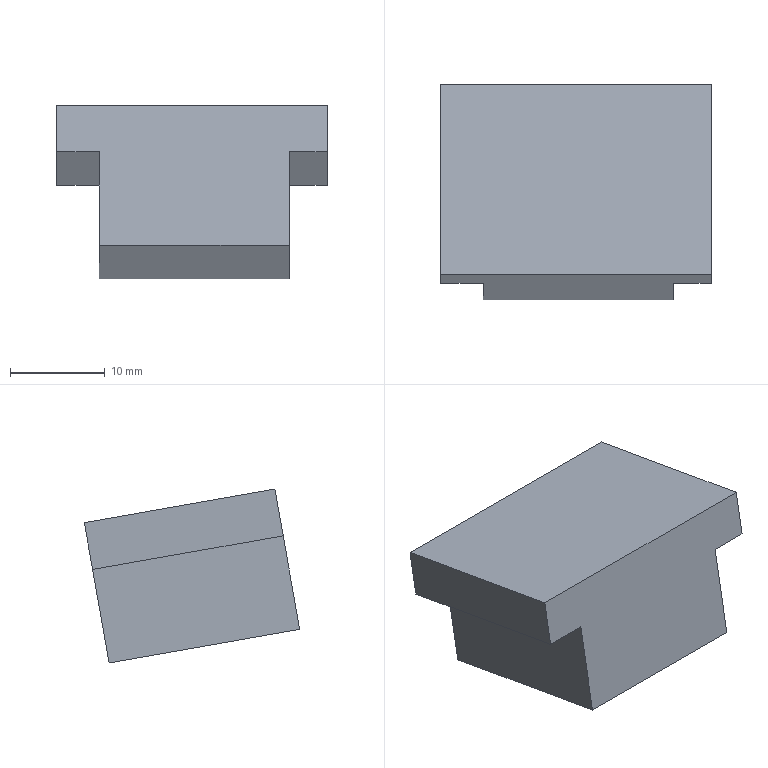Part | STEP file | 1 solid | 10 faces | box 28.5 x 22.681 x 18.312 mm | volume 6982 mm3 | plane 10
STEP:
#1=CARTESIAN_POINT('',(0.,0.,0.));
#2=DIRECTION('',(0.,0.,1.));
#3=DIRECTION('',(1.,0.,0.));
#4=AXIS2_PLACEMENT_3D('',#1,#2,#3);
#5=CARTESIAN_POINT('',(-28.862,49.056,-74.558));
#6=VERTEX_POINT('',#5);
#7=CARTESIAN_POINT('',(-32.862,49.056,-74.558));
#8=VERTEX_POINT('',#7);
#9=CARTESIAN_POINT('',(-43.112,49.056,-74.558));
#10=DIRECTION('',(-1.,0.,0.));
#11=VECTOR('',#10,1.);
#12=LINE('',#9,#11);
#13=CARTESIAN_POINT('',(-42.862,55.937,-75.771));
#14=DIRECTION('',(0.,-0.1736,-0.9848));
#15=DIRECTION('',(0.,0.9848,-0.1736));
#16=AXIS2_PLACEMENT_3D('',#13,#14,#15);
#17=PLANE('',#16);
#18=CARTESIAN_POINT('',(-6.987,-0.25));
#19=DIRECTION('',(0.,-1.));
#20=VECTOR('',#19,1.);
#21=LINE('',#18,#20);
#22=(GEOMETRIC_REPRESENTATION_CONTEXT(2)PARAMETRIC_REPRESENTATION_CONTEXT()REPRESENTATION_CONTEXT('',''));
#23=DEFINITIONAL_REPRESENTATION('',(#21),#22);
#24=PCURVE('',#17,#23);
#25=CARTESIAN_POINT('',(-43.112,49.924,-69.634));
#26=DIRECTION('',(0.,-0.9848,0.1736));
#27=DIRECTION('',(0.,-0.1736,-0.9848));
#28=AXIS2_PLACEMENT_3D('',#25,#26,#27);
#29=PLANE('',#28);
#30=CARTESIAN_POINT('',(5.,0.));
#31=DIRECTION('',(0.,-1.));
#32=VECTOR('',#31,1.);
#33=LINE('',#30,#32);
#34=(GEOMETRIC_REPRESENTATION_CONTEXT(2)PARAMETRIC_REPRESENTATION_CONTEXT()REPRESENTATION_CONTEXT('',''));
#35=DEFINITIONAL_REPRESENTATION('',(#33),#34);
#36=PCURVE('',#29,#35);
#37=SURFACE_CURVE('',#12,(#24,#36),.PCURVE_S1.);
#38=EDGE_CURVE('',#6,#8,#37,.T.);
#39=ORIENTED_EDGE('',*,*,#38,.T.);
#40=CARTESIAN_POINT('',(-32.862,69.132,-78.097));
#41=VERTEX_POINT('',#40);
#42=CARTESIAN_POINT('',(-32.862,4.542,-66.709));
#43=DIRECTION('',(0.,0.9848,-0.1736));
#44=VECTOR('',#43,1.);
#45=LINE('',#42,#44);
#46=CARTESIAN_POINT('',(-52.187,10.));
#47=DIRECTION('',(1.,0.));
#48=VECTOR('',#47,1.);
#49=LINE('',#46,#48);
#50=(GEOMETRIC_REPRESENTATION_CONTEXT(2)PARAMETRIC_REPRESENTATION_CONTEXT()REPRESENTATION_CONTEXT('',''));
#51=DEFINITIONAL_REPRESENTATION('',(#49),#50);
#52=PCURVE('',#17,#51);
#53=CARTESIAN_POINT('',(-32.862,0.,-92.47));
#54=DIRECTION('',(1.,0.,0.));
#55=DIRECTION('',(0.,0.,-1.));
#56=AXIS2_PLACEMENT_3D('',#53,#54,#55);
#57=PLANE('',#56);
#58=CARTESIAN_POINT('',(-25.762,4.542));
#59=DIRECTION('',(0.1736,0.9848));
#60=VECTOR('',#59,1.);
#61=LINE('',#58,#60);
#62=(GEOMETRIC_REPRESENTATION_CONTEXT(2)PARAMETRIC_REPRESENTATION_CONTEXT()REPRESENTATION_CONTEXT('',''));
#63=DEFINITIONAL_REPRESENTATION('',(#61),#62);
#64=PCURVE('',#57,#63);
#65=SURFACE_CURVE('',#45,(#52,#64),.PCURVE_S1.);
#66=EDGE_CURVE('',#8,#41,#65,.T.);
#67=ORIENTED_EDGE('',*,*,#66,.T.);
#68=CARTESIAN_POINT('',(-28.862,69.132,-78.097));
#69=VERTEX_POINT('',#68);
#70=CARTESIAN_POINT('',(-43.112,69.132,-78.097));
#71=DIRECTION('',(-1.,0.,0.));
#72=VECTOR('',#71,1.);
#73=LINE('',#70,#72);
#74=CARTESIAN_POINT('',(13.398,-0.25));
#75=DIRECTION('',(0.,-1.));
#76=VECTOR('',#75,1.);
#77=LINE('',#74,#76);
#78=(GEOMETRIC_REPRESENTATION_CONTEXT(2)PARAMETRIC_REPRESENTATION_CONTEXT()REPRESENTATION_CONTEXT('',''));
#79=DEFINITIONAL_REPRESENTATION('',(#77),#78);
#80=PCURVE('',#17,#79);
#81=CARTESIAN_POINT('',(-43.112,70.,-73.173));
#82=DIRECTION('',(0.,0.9848,-0.1736));
#83=DIRECTION('',(0.,0.1736,0.9848));
#84=AXIS2_PLACEMENT_3D('',#81,#82,#83);
#85=PLANE('',#84);
#86=CARTESIAN_POINT('',(-5.,0.));
#87=DIRECTION('',(0.,-1.));
#88=VECTOR('',#87,1.);
#89=LINE('',#86,#88);
#90=(GEOMETRIC_REPRESENTATION_CONTEXT(2)PARAMETRIC_REPRESENTATION_CONTEXT()REPRESENTATION_CONTEXT('',''));
#91=DEFINITIONAL_REPRESENTATION('',(#89),#90);
#92=PCURVE('',#85,#91);
#93=SURFACE_CURVE('',#73,(#80,#92),.PCURVE_S1.);
#94=EDGE_CURVE('',#69,#41,#93,.T.);
#95=ORIENTED_EDGE('',*,*,#94,.F.);
#96=CARTESIAN_POINT('',(-28.862,55.937,-75.771));
#97=DIRECTION('',(0.,-0.9848,0.1736));
#98=VECTOR('',#97,1.);
#99=LINE('',#96,#98);
#100=CARTESIAN_POINT('',(0.,14.));
#101=DIRECTION('',(-1.,0.));
#102=VECTOR('',#101,1.);
#103=LINE('',#100,#102);
#104=(GEOMETRIC_REPRESENTATION_CONTEXT(2)PARAMETRIC_REPRESENTATION_CONTEXT()REPRESENTATION_CONTEXT('',''));
#105=DEFINITIONAL_REPRESENTATION('',(#103),#104);
#106=PCURVE('',#17,#105);
#107=CARTESIAN_POINT('',(-28.862,57.5,-78.156));
#108=DIRECTION('',(1.,0.,0.));
#109=DIRECTION('',(0.,0.,-1.));
#110=AXIS2_PLACEMENT_3D('',#107,#108,#109);
#111=PLANE('',#110);
#112=CARTESIAN_POINT('',(-2.385,-1.563));
#113=DIRECTION('',(-0.1736,-0.9848));
#114=VECTOR('',#113,1.);
#115=LINE('',#112,#114);
#116=(GEOMETRIC_REPRESENTATION_CONTEXT(2)PARAMETRIC_REPRESENTATION_CONTEXT()REPRESENTATION_CONTEXT('',''));
#117=DEFINITIONAL_REPRESENTATION('',(#115),#116);
#118=PCURVE('',#111,#117);
#119=SURFACE_CURVE('',#99,(#106,#118),.PCURVE_S1.);
#120=EDGE_CURVE('',#69,#6,#119,.T.);
#121=ORIENTED_EDGE('',*,*,#120,.T.);
#122=EDGE_LOOP('',(#39,#67,#95,#121));
#123=FACE_BOUND('',#122,.T.);
#124=ADVANCED_FACE('',(#123),#17,.T.);
#125=CARTESIAN_POINT('',(-52.862,69.132,-78.097));
#126=VERTEX_POINT('',#125);
#127=CARTESIAN_POINT('',(-57.362,69.132,-78.097));
#128=VERTEX_POINT('',#127);
#129=CARTESIAN_POINT('',(-43.112,69.132,-78.097));
#130=DIRECTION('',(-1.,0.,0.));
#131=VECTOR('',#130,1.);
#132=LINE('',#129,#131);
#133=CARTESIAN_POINT('',(-42.862,55.937,-75.771));
#134=DIRECTION('',(0.,-0.1736,-0.9848));
#135=DIRECTION('',(0.,0.9848,-0.1736));
#136=AXIS2_PLACEMENT_3D('',#133,#134,#135);
#137=PLANE('',#136);
#138=CARTESIAN_POINT('',(13.398,-0.25));
#139=DIRECTION('',(0.,-1.));
#140=VECTOR('',#139,1.);
#141=LINE('',#138,#140);
#142=(GEOMETRIC_REPRESENTATION_CONTEXT(2)PARAMETRIC_REPRESENTATION_CONTEXT()REPRESENTATION_CONTEXT('',''));
#143=DEFINITIONAL_REPRESENTATION('',(#141),#142);
#144=PCURVE('',#137,#143);
#145=CARTESIAN_POINT('',(-5.,0.));
#146=DIRECTION('',(0.,-1.));
#147=VECTOR('',#146,1.);
#148=LINE('',#145,#147);
#149=(GEOMETRIC_REPRESENTATION_CONTEXT(2)PARAMETRIC_REPRESENTATION_CONTEXT()REPRESENTATION_CONTEXT('',''));
#150=DEFINITIONAL_REPRESENTATION('',(#148),#149);
#151=PCURVE('',#85,#150);
#152=SURFACE_CURVE('',#132,(#144,#151),.PCURVE_S1.);
#153=EDGE_CURVE('',#126,#128,#152,.T.);
#154=ORIENTED_EDGE('',*,*,#153,.F.);
#155=CARTESIAN_POINT('',(-52.862,49.056,-74.558));
#156=VERTEX_POINT('',#155);
#157=CARTESIAN_POINT('',(-52.862,4.542,-66.709));
#158=DIRECTION('',(0.,-0.9848,0.1736));
#159=VECTOR('',#158,1.);
#160=LINE('',#157,#159);
#161=CARTESIAN_POINT('',(-52.187,-10.));
#162=DIRECTION('',(-1.,0.));
#163=VECTOR('',#162,1.);
#164=LINE('',#161,#163);
#165=(GEOMETRIC_REPRESENTATION_CONTEXT(2)PARAMETRIC_REPRESENTATION_CONTEXT()REPRESENTATION_CONTEXT('',''));
#166=DEFINITIONAL_REPRESENTATION('',(#164),#165);
#167=PCURVE('',#137,#166);
#168=CARTESIAN_POINT('',(-52.862,0.,-92.47));
#169=DIRECTION('',(-1.,0.,0.));
#170=DIRECTION('',(0.,0.,1.));
#171=AXIS2_PLACEMENT_3D('',#168,#169,#170);
#172=PLANE('',#171);
#173=CARTESIAN_POINT('',(25.762,4.542));
#174=DIRECTION('',(0.1736,-0.9848));
#175=VECTOR('',#174,1.);
#176=LINE('',#173,#175);
#177=(GEOMETRIC_REPRESENTATION_CONTEXT(2)PARAMETRIC_REPRESENTATION_CONTEXT()REPRESENTATION_CONTEXT('',''));
#178=DEFINITIONAL_REPRESENTATION('',(#176),#177);
#179=PCURVE('',#172,#178);
#180=SURFACE_CURVE('',#160,(#167,#179),.PCURVE_S1.);
#181=EDGE_CURVE('',#126,#156,#180,.T.);
#182=ORIENTED_EDGE('',*,*,#181,.T.);
#183=CARTESIAN_POINT('',(-57.362,49.056,-74.558));
#184=VERTEX_POINT('',#183);
#185=CARTESIAN_POINT('',(-43.112,49.056,-74.558));
#186=DIRECTION('',(-1.,0.,0.));
#187=VECTOR('',#186,1.);
#188=LINE('',#185,#187);
#189=CARTESIAN_POINT('',(-6.987,-0.25));
#190=DIRECTION('',(0.,-1.));
#191=VECTOR('',#190,1.);
#192=LINE('',#189,#191);
#193=(GEOMETRIC_REPRESENTATION_CONTEXT(2)PARAMETRIC_REPRESENTATION_CONTEXT()REPRESENTATION_CONTEXT('',''));
#194=DEFINITIONAL_REPRESENTATION('',(#192),#193);
#195=PCURVE('',#137,#194);
#196=CARTESIAN_POINT('',(5.,0.));
#197=DIRECTION('',(0.,-1.));
#198=VECTOR('',#197,1.);
#199=LINE('',#196,#198);
#200=(GEOMETRIC_REPRESENTATION_CONTEXT(2)PARAMETRIC_REPRESENTATION_CONTEXT()REPRESENTATION_CONTEXT('',''));
#201=DEFINITIONAL_REPRESENTATION('',(#199),#200);
#202=PCURVE('',#29,#201);
#203=SURFACE_CURVE('',#188,(#195,#202),.PCURVE_S1.);
#204=EDGE_CURVE('',#156,#184,#203,.T.);
#205=ORIENTED_EDGE('',*,*,#204,.T.);
#206=CARTESIAN_POINT('',(-57.362,55.937,-75.771));
#207=DIRECTION('',(0.,0.9848,-0.1736));
#208=VECTOR('',#207,1.);
#209=LINE('',#206,#208);
#210=CARTESIAN_POINT('',(0.,-14.5));
#211=DIRECTION('',(1.,0.));
#212=VECTOR('',#211,1.);
#213=LINE('',#210,#212);
#214=(GEOMETRIC_REPRESENTATION_CONTEXT(2)PARAMETRIC_REPRESENTATION_CONTEXT()REPRESENTATION_CONTEXT('',''));
#215=DEFINITIONAL_REPRESENTATION('',(#213),#214);
#216=PCURVE('',#137,#215);
#217=CARTESIAN_POINT('',(-57.362,57.5,-78.156));
#218=DIRECTION('',(-1.,0.,0.));
#219=DIRECTION('',(0.,0.,1.));
#220=AXIS2_PLACEMENT_3D('',#217,#218,#219);
#221=PLANE('',#220);
#222=CARTESIAN_POINT('',(2.385,-1.563));
#223=DIRECTION('',(-0.1736,0.9848));
#224=VECTOR('',#223,1.);
#225=LINE('',#222,#224);
#226=(GEOMETRIC_REPRESENTATION_CONTEXT(2)PARAMETRIC_REPRESENTATION_CONTEXT()REPRESENTATION_CONTEXT('',''));
#227=DEFINITIONAL_REPRESENTATION('',(#225),#226);
#228=PCURVE('',#221,#227);
#229=SURFACE_CURVE('',#209,(#216,#228),.PCURVE_S1.);
#230=EDGE_CURVE('',#184,#128,#229,.T.);
#231=ORIENTED_EDGE('',*,*,#230,.T.);
#232=EDGE_LOOP('',(#154,#182,#205,#231));
#233=FACE_BOUND('',#232,.T.);
#234=ADVANCED_FACE('',(#233),#137,.T.);
#235=ORIENTED_EDGE('',*,*,#94,.T.);
#236=CARTESIAN_POINT('',(-32.862,67.395,-87.946));
#237=VERTEX_POINT('',#236);
#238=CARTESIAN_POINT('',(-32.862,64.589,-103.859));
#239=DIRECTION('',(0.,0.1736,0.9848));
#240=VECTOR('',#239,1.);
#241=LINE('',#238,#240);
#242=CARTESIAN_POINT('',(-31.159,10.25));
#243=DIRECTION('',(1.,0.));
#244=VECTOR('',#243,1.);
#245=LINE('',#242,#244);
#246=(GEOMETRIC_REPRESENTATION_CONTEXT(2)PARAMETRIC_REPRESENTATION_CONTEXT()REPRESENTATION_CONTEXT('',''));
#247=DEFINITIONAL_REPRESENTATION('',(#245),#246);
#248=PCURVE('',#85,#247);
#249=CARTESIAN_POINT('',(11.389,64.589));
#250=DIRECTION('',(-0.9848,0.1736));
#251=VECTOR('',#250,1.);
#252=LINE('',#249,#251);
#253=(GEOMETRIC_REPRESENTATION_CONTEXT(2)PARAMETRIC_REPRESENTATION_CONTEXT()REPRESENTATION_CONTEXT('',''));
#254=DEFINITIONAL_REPRESENTATION('',(#252),#253);
#255=PCURVE('',#57,#254);
#256=SURFACE_CURVE('',#241,(#248,#255),.PCURVE_S1.);
#257=EDGE_CURVE('',#237,#41,#256,.T.);
#258=ORIENTED_EDGE('',*,*,#257,.F.);
#259=CARTESIAN_POINT('',(-52.862,67.395,-87.946));
#260=VERTEX_POINT('',#259);
#261=CARTESIAN_POINT('',(-43.112,67.395,-87.946));
#262=DIRECTION('',(-1.,0.,0.));
#263=VECTOR('',#262,1.);
#264=LINE('',#261,#263);
#265=CARTESIAN_POINT('',(-15.,0.));
#266=DIRECTION('',(0.,-1.));
#267=VECTOR('',#266,1.);
#268=LINE('',#265,#267);
#269=(GEOMETRIC_REPRESENTATION_CONTEXT(2)PARAMETRIC_REPRESENTATION_CONTEXT()REPRESENTATION_CONTEXT('',''));
#270=DEFINITIONAL_REPRESENTATION('',(#268),#269);
#271=PCURVE('',#85,#270);
#272=CARTESIAN_POINT('',(-7.863,44.132,-83.844));
#273=DIRECTION('',(0.,0.1736,0.9848));
#274=DIRECTION('',(0.,-0.9848,0.1736));
#275=AXIS2_PLACEMENT_3D('',#272,#273,#274);
#276=PLANE('',#275);
#277=CARTESIAN_POINT('',(-23.622,-35.25));
#278=DIRECTION('',(0.,-1.));
#279=VECTOR('',#278,1.);
#280=LINE('',#277,#279);
#281=(GEOMETRIC_REPRESENTATION_CONTEXT(2)PARAMETRIC_REPRESENTATION_CONTEXT()REPRESENTATION_CONTEXT('',''));
#282=DEFINITIONAL_REPRESENTATION('',(#280),#281);
#283=PCURVE('',#276,#282);
#284=SURFACE_CURVE('',#264,(#271,#283),.PCURVE_S1.);
#285=EDGE_CURVE('',#237,#260,#284,.T.);
#286=ORIENTED_EDGE('',*,*,#285,.T.);
#287=CARTESIAN_POINT('',(-52.862,70.,-73.173));
#288=DIRECTION('',(0.,0.1736,0.9848));
#289=VECTOR('',#288,1.);
#290=LINE('',#287,#289);
#291=CARTESIAN_POINT('',(0.,-9.75));
#292=DIRECTION('',(1.,0.));
#293=VECTOR('',#292,1.);
#294=LINE('',#291,#293);
#295=(GEOMETRIC_REPRESENTATION_CONTEXT(2)PARAMETRIC_REPRESENTATION_CONTEXT()REPRESENTATION_CONTEXT('',''));
#296=DEFINITIONAL_REPRESENTATION('',(#294),#295);
#297=PCURVE('',#85,#296);
#298=CARTESIAN_POINT('',(19.297,70.));
#299=DIRECTION('',(0.9848,0.1736));
#300=VECTOR('',#299,1.);
#301=LINE('',#298,#300);
#302=(GEOMETRIC_REPRESENTATION_CONTEXT(2)PARAMETRIC_REPRESENTATION_CONTEXT()REPRESENTATION_CONTEXT('',''));
#303=DEFINITIONAL_REPRESENTATION('',(#301),#302);
#304=PCURVE('',#172,#303);
#305=SURFACE_CURVE('',#290,(#297,#304),.PCURVE_S1.);
#306=EDGE_CURVE('',#260,#126,#305,.T.);
#307=ORIENTED_EDGE('',*,*,#306,.T.);
#308=ORIENTED_EDGE('',*,*,#153,.T.);
#309=CARTESIAN_POINT('',(-57.362,70.,-73.173));
#310=VERTEX_POINT('',#309);
#311=CARTESIAN_POINT('',(-57.362,70.,-73.173));
#312=DIRECTION('',(0.,0.1736,0.9848));
#313=VECTOR('',#312,1.);
#314=LINE('',#311,#313);
#315=CARTESIAN_POINT('',(0.,-14.25));
#316=DIRECTION('',(1.,0.));
#317=VECTOR('',#316,1.);
#318=LINE('',#315,#317);
#319=(GEOMETRIC_REPRESENTATION_CONTEXT(2)PARAMETRIC_REPRESENTATION_CONTEXT()REPRESENTATION_CONTEXT('',''));
#320=DEFINITIONAL_REPRESENTATION('',(#318),#319);
#321=PCURVE('',#85,#320);
#322=CARTESIAN_POINT('',(4.983,12.5));
#323=DIRECTION('',(0.9848,0.1736));
#324=VECTOR('',#323,1.);
#325=LINE('',#322,#324);
#326=(GEOMETRIC_REPRESENTATION_CONTEXT(2)PARAMETRIC_REPRESENTATION_CONTEXT()REPRESENTATION_CONTEXT('',''));
#327=DEFINITIONAL_REPRESENTATION('',(#325),#326);
#328=PCURVE('',#221,#327);
#329=SURFACE_CURVE('',#314,(#321,#328),.PCURVE_S1.);
#330=EDGE_CURVE('',#128,#310,#329,.T.);
#331=ORIENTED_EDGE('',*,*,#330,.T.);
#332=CARTESIAN_POINT('',(-28.862,70.,-73.173));
#333=VERTEX_POINT('',#332);
#334=CARTESIAN_POINT('',(-43.112,70.,-73.173));
#335=DIRECTION('',(-1.,0.,0.));
#336=VECTOR('',#335,1.);
#337=LINE('',#334,#336);
#338=CARTESIAN_POINT('',(0.,0.));
#339=DIRECTION('',(0.,-1.));
#340=VECTOR('',#339,1.);
#341=LINE('',#338,#340);
#342=(GEOMETRIC_REPRESENTATION_CONTEXT(2)PARAMETRIC_REPRESENTATION_CONTEXT()REPRESENTATION_CONTEXT('',''));
#343=DEFINITIONAL_REPRESENTATION('',(#341),#342);
#344=PCURVE('',#85,#343);
#345=CARTESIAN_POINT('',(-42.862,58.368,-71.122));
#346=DIRECTION('',(0.,-0.1736,-0.9848));
#347=DIRECTION('',(0.,0.9848,-0.1736));
#348=AXIS2_PLACEMENT_3D('',#345,#346,#347);
#349=PLANE('',#348);
#350=CARTESIAN_POINT('',(11.811,-0.25));
#351=DIRECTION('',(0.,-1.));
#352=VECTOR('',#351,1.);
#353=LINE('',#350,#352);
#354=(GEOMETRIC_REPRESENTATION_CONTEXT(2)PARAMETRIC_REPRESENTATION_CONTEXT()REPRESENTATION_CONTEXT('',''));
#355=DEFINITIONAL_REPRESENTATION('',(#353),#354);
#356=PCURVE('',#349,#355);
#357=SURFACE_CURVE('',#337,(#344,#356),.PCURVE_S1.);
#358=EDGE_CURVE('',#333,#310,#357,.T.);
#359=ORIENTED_EDGE('',*,*,#358,.F.);
#360=CARTESIAN_POINT('',(-28.862,70.,-73.173));
#361=DIRECTION('',(0.,-0.1736,-0.9848));
#362=VECTOR('',#361,1.);
#363=LINE('',#360,#362);
#364=CARTESIAN_POINT('',(0.,14.25));
#365=DIRECTION('',(-1.,0.));
#366=VECTOR('',#365,1.);
#367=LINE('',#364,#366);
#368=(GEOMETRIC_REPRESENTATION_CONTEXT(2)PARAMETRIC_REPRESENTATION_CONTEXT()REPRESENTATION_CONTEXT('',''));
#369=DEFINITIONAL_REPRESENTATION('',(#367),#368);
#370=PCURVE('',#85,#369);
#371=CARTESIAN_POINT('',(-4.983,12.5));
#372=DIRECTION('',(0.9848,-0.1736));
#373=VECTOR('',#372,1.);
#374=LINE('',#371,#373);
#375=(GEOMETRIC_REPRESENTATION_CONTEXT(2)PARAMETRIC_REPRESENTATION_CONTEXT()REPRESENTATION_CONTEXT('',''));
#376=DEFINITIONAL_REPRESENTATION('',(#374),#375);
#377=PCURVE('',#111,#376);
#378=SURFACE_CURVE('',#363,(#370,#377),.PCURVE_S1.);
#379=EDGE_CURVE('',#333,#69,#378,.T.);
#380=ORIENTED_EDGE('',*,*,#379,.T.);
#381=EDGE_LOOP('',(#235,#258,#286,#307,#308,#331,#359,#380));
#382=FACE_BOUND('',#381,.T.);
#383=ADVANCED_FACE('',(#382),#85,.T.);
#384=CARTESIAN_POINT('',(-57.362,49.924,-69.634));
#385=VERTEX_POINT('',#384);
#386=CARTESIAN_POINT('',(-57.362,49.924,-69.634));
#387=DIRECTION('',(0.,0.1736,0.9848));
#388=VECTOR('',#387,1.);
#389=LINE('',#386,#388);
#390=CARTESIAN_POINT('',(0.,-14.25));
#391=DIRECTION('',(-1.,0.));
#392=VECTOR('',#391,1.);
#393=LINE('',#390,#392);
#394=(GEOMETRIC_REPRESENTATION_CONTEXT(2)PARAMETRIC_REPRESENTATION_CONTEXT()REPRESENTATION_CONTEXT('',''));
#395=DEFINITIONAL_REPRESENTATION('',(#393),#394);
#396=PCURVE('',#29,#395);
#397=CARTESIAN_POINT('',(8.523,-7.576));
#398=DIRECTION('',(0.9848,0.1736));
#399=VECTOR('',#398,1.);
#400=LINE('',#397,#399);
#401=(GEOMETRIC_REPRESENTATION_CONTEXT(2)PARAMETRIC_REPRESENTATION_CONTEXT()REPRESENTATION_CONTEXT('',''));
#402=DEFINITIONAL_REPRESENTATION('',(#400),#401);
#403=PCURVE('',#221,#402);
#404=SURFACE_CURVE('',#389,(#396,#403),.PCURVE_S1.);
#405=EDGE_CURVE('',#184,#385,#404,.T.);
#406=ORIENTED_EDGE('',*,*,#405,.F.);
#407=ORIENTED_EDGE('',*,*,#204,.F.);
#408=CARTESIAN_POINT('',(-52.862,47.319,-84.406));
#409=VERTEX_POINT('',#408);
#410=CARTESIAN_POINT('',(-52.862,44.513,-100.319));
#411=DIRECTION('',(0.,-0.1736,-0.9848));
#412=VECTOR('',#411,1.);
#413=LINE('',#410,#412);
#414=CARTESIAN_POINT('',(31.159,-9.75));
#415=DIRECTION('',(1.,0.));
#416=VECTOR('',#415,1.);
#417=LINE('',#414,#416);
#418=(GEOMETRIC_REPRESENTATION_CONTEXT(2)PARAMETRIC_REPRESENTATION_CONTEXT()REPRESENTATION_CONTEXT('',''));
#419=DEFINITIONAL_REPRESENTATION('',(#417),#418);
#420=PCURVE('',#29,#419);
#421=CARTESIAN_POINT('',(-7.849,44.513));
#422=DIRECTION('',(-0.9848,-0.1736));
#423=VECTOR('',#422,1.);
#424=LINE('',#421,#423);
#425=(GEOMETRIC_REPRESENTATION_CONTEXT(2)PARAMETRIC_REPRESENTATION_CONTEXT()REPRESENTATION_CONTEXT('',''));
#426=DEFINITIONAL_REPRESENTATION('',(#424),#425);
#427=PCURVE('',#172,#426);
#428=SURFACE_CURVE('',#413,(#420,#427),.PCURVE_S1.);
#429=EDGE_CURVE('',#156,#409,#428,.T.);
#430=ORIENTED_EDGE('',*,*,#429,.T.);
#431=CARTESIAN_POINT('',(-32.862,47.319,-84.406));
#432=VERTEX_POINT('',#431);
#433=CARTESIAN_POINT('',(-43.112,47.319,-84.406));
#434=DIRECTION('',(-1.,0.,0.));
#435=VECTOR('',#434,1.);
#436=LINE('',#433,#435);
#437=CARTESIAN_POINT('',(15.,0.));
#438=DIRECTION('',(0.,-1.));
#439=VECTOR('',#438,1.);
#440=LINE('',#437,#439);
#441=(GEOMETRIC_REPRESENTATION_CONTEXT(2)PARAMETRIC_REPRESENTATION_CONTEXT()REPRESENTATION_CONTEXT('',''));
#442=DEFINITIONAL_REPRESENTATION('',(#440),#441);
#443=PCURVE('',#29,#442);
#444=CARTESIAN_POINT('',(-3.237,-35.25));
#445=DIRECTION('',(0.,-1.));
#446=VECTOR('',#445,1.);
#447=LINE('',#444,#446);
#448=(GEOMETRIC_REPRESENTATION_CONTEXT(2)PARAMETRIC_REPRESENTATION_CONTEXT()REPRESENTATION_CONTEXT('',''));
#449=DEFINITIONAL_REPRESENTATION('',(#447),#448);
#450=PCURVE('',#276,#449);
#451=SURFACE_CURVE('',#436,(#443,#450),.PCURVE_S1.);
#452=EDGE_CURVE('',#432,#409,#451,.T.);
#453=ORIENTED_EDGE('',*,*,#452,.F.);
#454=CARTESIAN_POINT('',(-32.862,44.513,-100.319));
#455=DIRECTION('',(0.,0.1736,0.9848));
#456=VECTOR('',#455,1.);
#457=LINE('',#454,#456);
#458=CARTESIAN_POINT('',(31.159,10.25));
#459=DIRECTION('',(-1.,0.));
#460=VECTOR('',#459,1.);
#461=LINE('',#458,#460);
#462=(GEOMETRIC_REPRESENTATION_CONTEXT(2)PARAMETRIC_REPRESENTATION_CONTEXT()REPRESENTATION_CONTEXT('',''));
#463=DEFINITIONAL_REPRESENTATION('',(#461),#462);
#464=PCURVE('',#29,#463);
#465=CARTESIAN_POINT('',(7.849,44.513));
#466=DIRECTION('',(-0.9848,0.1736));
#467=VECTOR('',#466,1.);
#468=LINE('',#465,#467);
#469=(GEOMETRIC_REPRESENTATION_CONTEXT(2)PARAMETRIC_REPRESENTATION_CONTEXT()REPRESENTATION_CONTEXT('',''));
#470=DEFINITIONAL_REPRESENTATION('',(#468),#469);
#471=PCURVE('',#57,#470);
#472=SURFACE_CURVE('',#457,(#464,#471),.PCURVE_S1.);
#473=EDGE_CURVE('',#432,#8,#472,.T.);
#474=ORIENTED_EDGE('',*,*,#473,.T.);
#475=ORIENTED_EDGE('',*,*,#38,.F.);
#476=CARTESIAN_POINT('',(-28.862,49.924,-69.634));
#477=VERTEX_POINT('',#476);
#478=CARTESIAN_POINT('',(-28.862,49.924,-69.634));
#479=DIRECTION('',(0.,-0.1736,-0.9848));
#480=VECTOR('',#479,1.);
#481=LINE('',#478,#480);
#482=CARTESIAN_POINT('',(0.,14.25));
#483=DIRECTION('',(1.,0.));
#484=VECTOR('',#483,1.);
#485=LINE('',#482,#484);
#486=(GEOMETRIC_REPRESENTATION_CONTEXT(2)PARAMETRIC_REPRESENTATION_CONTEXT()REPRESENTATION_CONTEXT('',''));
#487=DEFINITIONAL_REPRESENTATION('',(#485),#486);
#488=PCURVE('',#29,#487);
#489=CARTESIAN_POINT('',(-8.523,-7.576));
#490=DIRECTION('',(0.9848,-0.1736));
#491=VECTOR('',#490,1.);
#492=LINE('',#489,#491);
#493=(GEOMETRIC_REPRESENTATION_CONTEXT(2)PARAMETRIC_REPRESENTATION_CONTEXT()REPRESENTATION_CONTEXT('',''));
#494=DEFINITIONAL_REPRESENTATION('',(#492),#493);
#495=PCURVE('',#111,#494);
#496=SURFACE_CURVE('',#481,(#488,#495),.PCURVE_S1.);
#497=EDGE_CURVE('',#477,#6,#496,.T.);
#498=ORIENTED_EDGE('',*,*,#497,.F.);
#499=CARTESIAN_POINT('',(-43.112,49.924,-69.634));
#500=DIRECTION('',(-1.,0.,0.));
#501=VECTOR('',#500,1.);
#502=LINE('',#499,#501);
#503=CARTESIAN_POINT('',(0.,0.));
#504=DIRECTION('',(0.,-1.));
#505=VECTOR('',#504,1.);
#506=LINE('',#503,#505);
#507=(GEOMETRIC_REPRESENTATION_CONTEXT(2)PARAMETRIC_REPRESENTATION_CONTEXT()REPRESENTATION_CONTEXT('',''));
#508=DEFINITIONAL_REPRESENTATION('',(#506),#507);
#509=PCURVE('',#29,#508);
#510=CARTESIAN_POINT('',(-8.574,-0.25));
#511=DIRECTION('',(0.,-1.));
#512=VECTOR('',#511,1.);
#513=LINE('',#510,#512);
#514=(GEOMETRIC_REPRESENTATION_CONTEXT(2)PARAMETRIC_REPRESENTATION_CONTEXT()REPRESENTATION_CONTEXT('',''));
#515=DEFINITIONAL_REPRESENTATION('',(#513),#514);
#516=PCURVE('',#349,#515);
#517=SURFACE_CURVE('',#502,(#509,#516),.PCURVE_S1.);
#518=EDGE_CURVE('',#477,#385,#517,.T.);
#519=ORIENTED_EDGE('',*,*,#518,.T.);
#520=EDGE_LOOP('',(#406,#407,#430,#453,#474,#475,#498,#519));
#521=FACE_BOUND('',#520,.T.);
#522=ADVANCED_FACE('',(#521),#29,.T.);
#523=CARTESIAN_POINT('',(-57.362,58.368,-71.122));
#524=DIRECTION('',(0.,0.9848,-0.1736));
#525=VECTOR('',#524,1.);
#526=LINE('',#523,#525);
#527=CARTESIAN_POINT('',(0.,-14.5));
#528=DIRECTION('',(1.,0.));
#529=VECTOR('',#528,1.);
#530=LINE('',#527,#529);
#531=(GEOMETRIC_REPRESENTATION_CONTEXT(2)PARAMETRIC_REPRESENTATION_CONTEXT()REPRESENTATION_CONTEXT('',''));
#532=DEFINITIONAL_REPRESENTATION('',(#530),#531);
#533=PCURVE('',#349,#532);
#534=CARTESIAN_POINT('',(7.034,0.8682));
#535=DIRECTION('',(-0.1736,0.9848));
#536=VECTOR('',#535,1.);
#537=LINE('',#534,#536);
#538=(GEOMETRIC_REPRESENTATION_CONTEXT(2)PARAMETRIC_REPRESENTATION_CONTEXT()REPRESENTATION_CONTEXT('',''));
#539=DEFINITIONAL_REPRESENTATION('',(#537),#538);
#540=PCURVE('',#221,#539);
#541=SURFACE_CURVE('',#526,(#533,#540),.PCURVE_S1.);
#542=EDGE_CURVE('',#385,#310,#541,.T.);
#543=ORIENTED_EDGE('',*,*,#542,.F.);
#544=ORIENTED_EDGE('',*,*,#518,.F.);
#545=CARTESIAN_POINT('',(-28.862,58.368,-71.122));
#546=DIRECTION('',(0.,-0.9848,0.1736));
#547=VECTOR('',#546,1.);
#548=LINE('',#545,#547);
#549=CARTESIAN_POINT('',(0.,14.));
#550=DIRECTION('',(-1.,0.));
#551=VECTOR('',#550,1.);
#552=LINE('',#549,#551);
#553=(GEOMETRIC_REPRESENTATION_CONTEXT(2)PARAMETRIC_REPRESENTATION_CONTEXT()REPRESENTATION_CONTEXT('',''));
#554=DEFINITIONAL_REPRESENTATION('',(#552),#553);
#555=PCURVE('',#349,#554);
#556=CARTESIAN_POINT('',(-7.034,0.8682));
#557=DIRECTION('',(-0.1736,-0.9848));
#558=VECTOR('',#557,1.);
#559=LINE('',#556,#558);
#560=(GEOMETRIC_REPRESENTATION_CONTEXT(2)PARAMETRIC_REPRESENTATION_CONTEXT()REPRESENTATION_CONTEXT('',''));
#561=DEFINITIONAL_REPRESENTATION('',(#559),#560);
#562=PCURVE('',#111,#561);
#563=SURFACE_CURVE('',#548,(#555,#562),.PCURVE_S1.);
#564=EDGE_CURVE('',#333,#477,#563,.T.);
#565=ORIENTED_EDGE('',*,*,#564,.F.);
#566=ORIENTED_EDGE('',*,*,#358,.T.);
#567=EDGE_LOOP('',(#543,#544,#565,#566));
#568=FACE_BOUND('',#567,.T.);
#569=ADVANCED_FACE('',(#568),#349,.F.);
#570=ORIENTED_EDGE('',*,*,#120,.F.);
#571=ORIENTED_EDGE('',*,*,#379,.F.);
#572=ORIENTED_EDGE('',*,*,#564,.T.);
#573=ORIENTED_EDGE('',*,*,#497,.T.);
#574=EDGE_LOOP('',(#570,#571,#572,#573));
#575=FACE_BOUND('',#574,.T.);
#576=ADVANCED_FACE('',(#575),#111,.T.);
#577=ORIENTED_EDGE('',*,*,#230,.F.);
#578=ORIENTED_EDGE('',*,*,#405,.T.);
#579=ORIENTED_EDGE('',*,*,#542,.T.);
#580=ORIENTED_EDGE('',*,*,#330,.F.);
#581=EDGE_LOOP('',(#577,#578,#579,#580));
#582=FACE_BOUND('',#581,.T.);
#583=ADVANCED_FACE('',(#582),#221,.T.);
#584=ORIENTED_EDGE('',*,*,#452,.T.);
#585=CARTESIAN_POINT('',(-52.862,2.806,-76.557));
#586=DIRECTION('',(0.,-0.9848,0.1736));
#587=VECTOR('',#586,1.);
#588=LINE('',#585,#587);
#589=CARTESIAN_POINT('',(41.963,-45.));
#590=DIRECTION('',(1.,0.));
#591=VECTOR('',#590,1.);
#592=LINE('',#589,#591);
#593=(GEOMETRIC_REPRESENTATION_CONTEXT(2)PARAMETRIC_REPRESENTATION_CONTEXT()REPRESENTATION_CONTEXT('',''));
#594=DEFINITIONAL_REPRESENTATION('',(#592),#593);
#595=PCURVE('',#276,#594);
#596=CARTESIAN_POINT('',(15.914,2.806));
#597=DIRECTION('',(0.1736,-0.9848));
#598=VECTOR('',#597,1.);
#599=LINE('',#596,#598);
#600=(GEOMETRIC_REPRESENTATION_CONTEXT(2)PARAMETRIC_REPRESENTATION_CONTEXT()REPRESENTATION_CONTEXT('',''));
#601=DEFINITIONAL_REPRESENTATION('',(#599),#600);
#602=PCURVE('',#172,#601);
#603=SURFACE_CURVE('',#588,(#595,#602),.PCURVE_S1.);
#604=EDGE_CURVE('',#260,#409,#603,.T.);
#605=ORIENTED_EDGE('',*,*,#604,.F.);
#606=ORIENTED_EDGE('',*,*,#285,.F.);
#607=CARTESIAN_POINT('',(-32.862,2.806,-76.557));
#608=DIRECTION('',(0.,0.9848,-0.1736));
#609=VECTOR('',#608,1.);
#610=LINE('',#607,#609);
#611=CARTESIAN_POINT('',(41.963,-25.));
#612=DIRECTION('',(-1.,0.));
#613=VECTOR('',#612,1.);
#614=LINE('',#611,#613);
#615=(GEOMETRIC_REPRESENTATION_CONTEXT(2)PARAMETRIC_REPRESENTATION_CONTEXT()REPRESENTATION_CONTEXT('',''));
#616=DEFINITIONAL_REPRESENTATION('',(#614),#615);
#617=PCURVE('',#276,#616);
#618=CARTESIAN_POINT('',(-15.914,2.806));
#619=DIRECTION('',(0.1736,0.9848));
#620=VECTOR('',#619,1.);
#621=LINE('',#618,#620);
#622=(GEOMETRIC_REPRESENTATION_CONTEXT(2)PARAMETRIC_REPRESENTATION_CONTEXT()REPRESENTATION_CONTEXT('',''));
#623=DEFINITIONAL_REPRESENTATION('',(#621),#622);
#624=PCURVE('',#57,#623);
#625=SURFACE_CURVE('',#610,(#617,#624),.PCURVE_S1.);
#626=EDGE_CURVE('',#432,#237,#625,.T.);
#627=ORIENTED_EDGE('',*,*,#626,.F.);
#628=EDGE_LOOP('',(#584,#605,#606,#627));
#629=FACE_BOUND('',#628,.T.);
#630=ADVANCED_FACE('',(#629),#276,.F.);
#631=ORIENTED_EDGE('',*,*,#181,.F.);
#632=ORIENTED_EDGE('',*,*,#306,.F.);
#633=ORIENTED_EDGE('',*,*,#604,.T.);
#634=ORIENTED_EDGE('',*,*,#429,.F.);
#635=EDGE_LOOP('',(#631,#632,#633,#634));
#636=FACE_BOUND('',#635,.T.);
#637=ADVANCED_FACE('',(#636),#172,.T.);
#638=ORIENTED_EDGE('',*,*,#257,.T.);
#639=ORIENTED_EDGE('',*,*,#66,.F.);
#640=ORIENTED_EDGE('',*,*,#473,.F.);
#641=ORIENTED_EDGE('',*,*,#626,.T.);
#642=EDGE_LOOP('',(#638,#639,#640,#641));
#643=FACE_BOUND('',#642,.T.);
#644=ADVANCED_FACE('',(#643),#57,.T.);
#645=CLOSED_SHELL('',(#124,#234,#383,#522,#569,#576,#583,#630,#637,#644));
#646=MANIFOLD_SOLID_BREP('',#645);
#647=(LENGTH_UNIT()NAMED_UNIT(*)SI_UNIT(.MILLI.,.METRE.));
#648=UNCERTAINTY_MEASURE_WITH_UNIT(LENGTH_MEASURE(0.0000001),#647,'','');
#649=(NAMED_UNIT(*)PLANE_ANGLE_UNIT()SI_UNIT($,.RADIAN.));
#650=(NAMED_UNIT(*)SI_UNIT($,.STERADIAN.)SOLID_ANGLE_UNIT());
#651=(GEOMETRIC_REPRESENTATION_CONTEXT(3)GLOBAL_UNCERTAINTY_ASSIGNED_CONTEXT((#648))GLOBAL_UNIT_ASSIGNED_CONTEXT((#647,#649,#650))REPRESENTATION_CONTEXT('',''));
#652=ADVANCED_BREP_SHAPE_REPRESENTATION('',(#4,#646),#651);